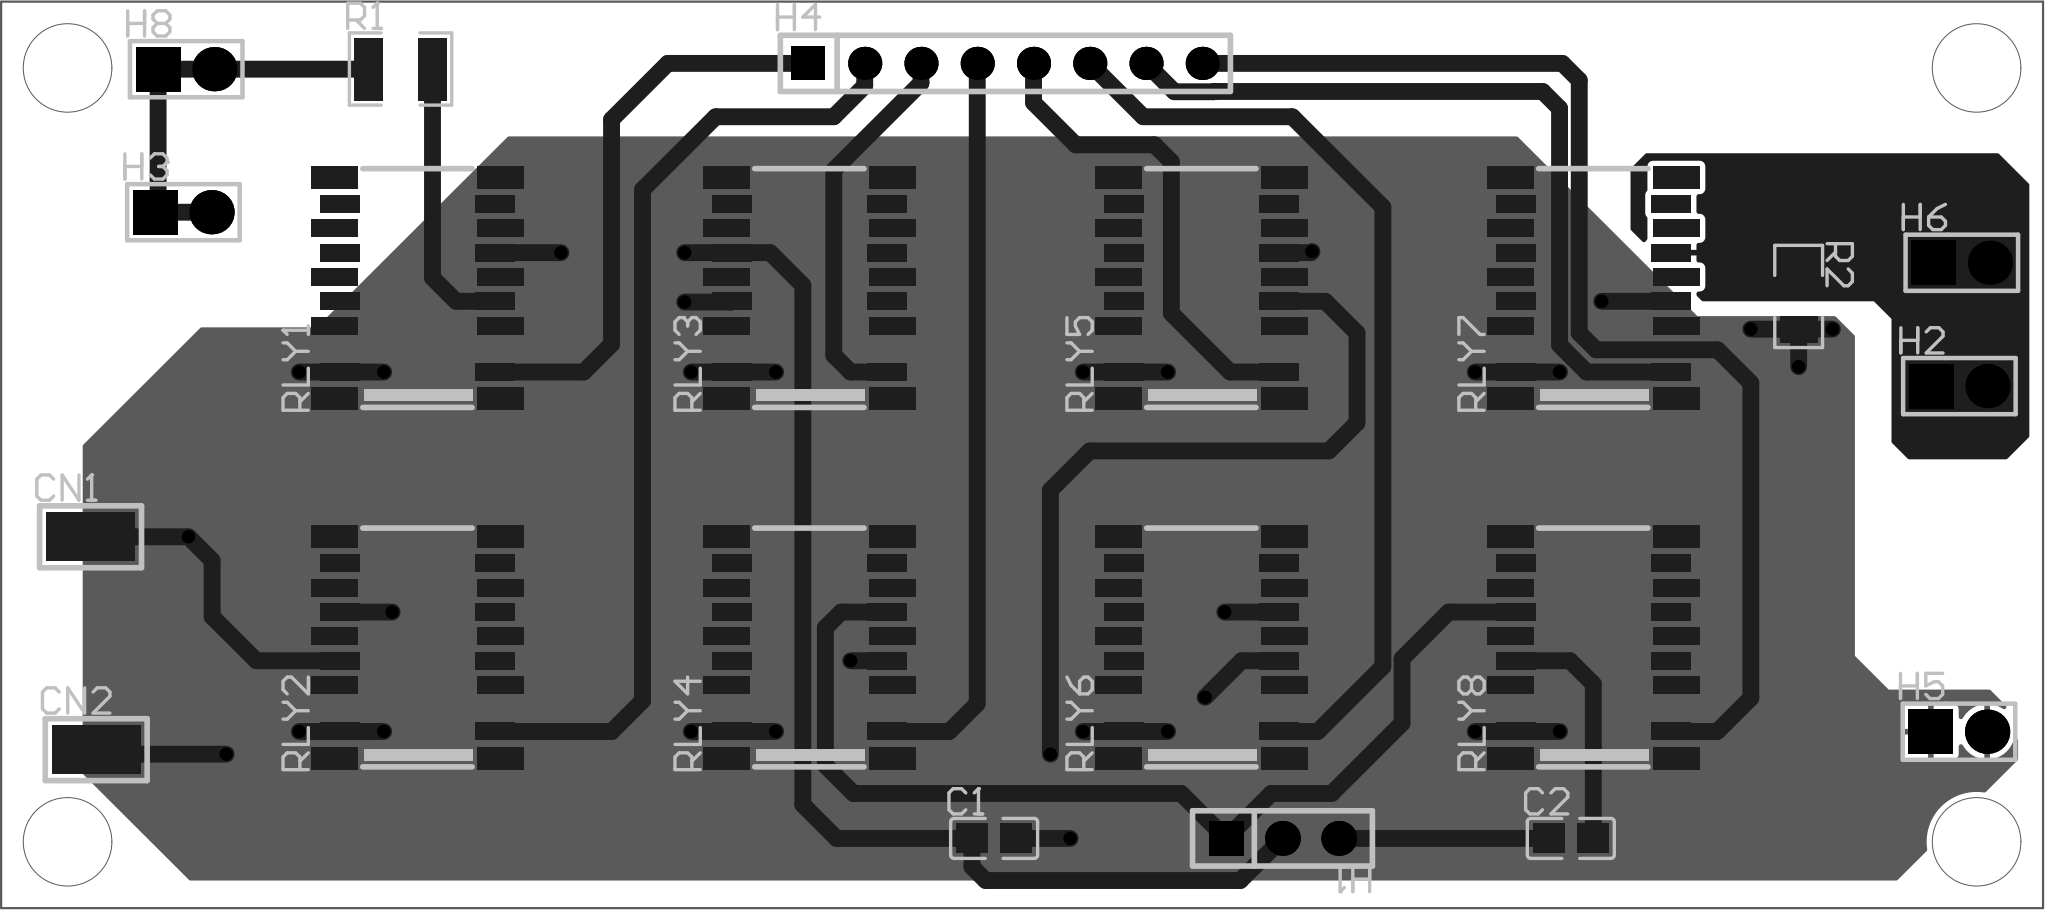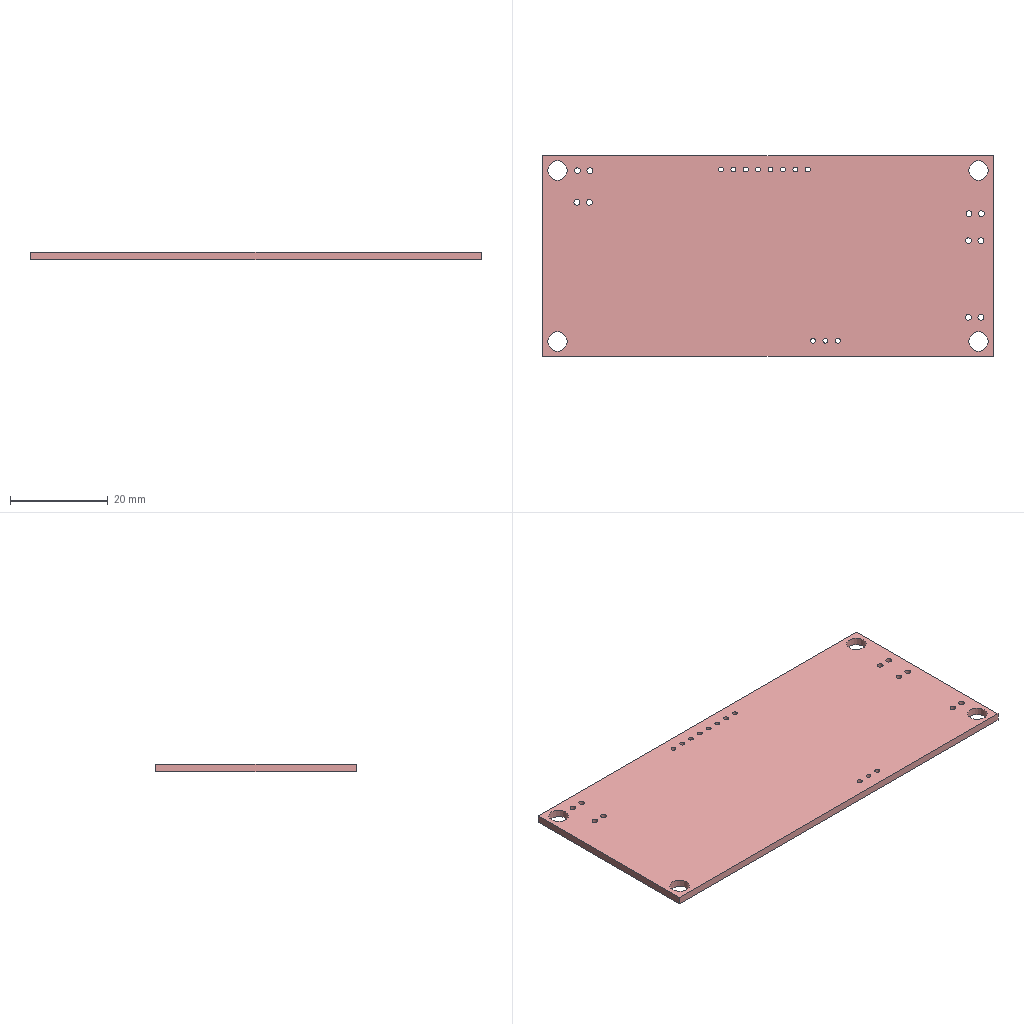Circuit board layout | Altium Designer | box 92.2 x 41 x 1.6 mm
Layer stack:
# Altium Designer layer stack of  (unit mm; dielectric type: 0 none, 1 core, 2 prepreg, 3 surface material)
index,name,kind,layer,copper_thickness_mm,dielectric_type,dielectric_thickness_mm,dielectric_material,dielectric_constant
0,Top Paste Mask Layer,other,,,,,,
1,Top Silkscreen Layer,other,,,,,,
2,Top Solder Mask Layer,dielectric,,,3,0.01,,3.3
3,Top Layer,copper,Top Layer,0.035,,,,
4,Dielectric1,dielectric,,,3,1.51,FR4,4.5
5,Bottom Layer,copper,Bottom Layer,0.035,,,,
6,Bottom Solder Mask Layer,dielectric,,,3,0.01,,3.3
7,Bottom Silkscreen Layer,other,,,,,,
8,Bottom Paste Mask Layer,other,,,,,,
# drill layer pairs: low layer,high layer
drill_pair,Top Layer,Bottom Layer
Part placement:
Designator,Comment,Layer,Footprint,Center-X(mm),Center-Y(mm),Rotation
C1,470nF,TopLayer,C0805,121.031,79.354,0
C2,470nF,TopLayer,C0805,147.066,79.354,0
CN1,RH-5019,TopLayer,TESTPOINT-SMD_L3.8-W2.0_RH-5019,80.239,92.995,0
CN2,RH-5019,TopLayer,TESTPOINT-SMD_L3.8-W2.0_RH-5019,80.493,83.368,0
H1,PM254V-11-03-H85,TopLayer,HDR-TH_3P-P2.54-V-F,134.048,79.354,0
H2,PZ254V-11-02P,TopLayer,HDR-TH_2P-P2.54-V-M,164.609,99.811,0
H3,PZ254V-11-02P,TopLayer,HDR-TH_2P-P2.54-V-M,84.43,107.675,0
H4,PZ254V-11-08P,TopLayer,HDR-TH_8P-P2.54-V-M,121.539,114.406,0
H5,PZ254V-11-02P,TopLayer,HDR-TH_2P-P2.54-V-M,164.592,84.18,0
H6,PZ254V-11-02P,TopLayer,HDR-TH_2P-P2.54-V-M,164.719,105.389,0
H8,PZ254V-11-02P,TopLayer,HDR-TH_2P-P2.54-V-M,84.557,114.144,0
R1,1kΩ,TopLayer,R1210,94.234,114.152,0
R2,0Ω,TopLayer,R1206,157.353,103.865,270
RLY1,G6K-2F-RF-S DC5,TopLayer,RELAY-SMD_G6K-2F-RF-S-DC12,94.996,104.246,90
RLY2,G6K-2F-RF-S DC5,TopLayer,RELAY-SMD_G6K-2F-RF-S-DC12,94.996,87.99,90
RLY3,G6K-2F-RF-S DC5,TopLayer,RELAY-SMD_G6K-2F-RF-S-DC12,112.691,104.246,90
RLY4,G6K-2F-RF-S DC5,TopLayer,RELAY-SMD_G6K-2F-RF-S-DC12,112.691,87.99,90
RLY5,G6K-2F-RF-S DC5,TopLayer,RELAY-SMD_G6K-2F-RF-S-DC12,130.387,104.246,90
RLY6,G6K-2F-RF-S DC5,TopLayer,RELAY-SMD_G6K-2F-RF-S-DC12,130.387,87.99,90
RLY7,G6K-2F-RF-S DC5,TopLayer,RELAY-SMD_G6K-2F-RF-S-DC12,148.082,104.246,90
RLY8,G6K-2F-RF-S DC5,TopLayer,RELAY-SMD_G6K-2F-RF-S-DC12,148.082,87.99,90
Pad and via stacks:
# Altium Designer via and pad stacks of  (unit mm). Each distinct definition once, with the count of objects using it.
# via: kind,start_layer,end_layer,hole_mm,diameter_mm,mode(0 simple;1 top-mid-bottom;2 full stack),diameter_per_layer,count,example_net
# pad: kind,layer,hole_mm,hole_type(0 round;1 square;2 slot),plating,top_size,top_shape(1 round;2 rect;3 octagon;9 rounded rect),mid_size,bottom_size,mode,footprint,size_per_layer,count,example
pad,Top Layer,0,0,plated,1.41x1.35,2,1.41x1.35,1.41x1.35,0,C0805,,4,C1.2
pad,Top Layer,0,0,plated,4x2.2,2,4x2.2,4x2.2,0,TESTPOINT-SMD_L3.8-W2.0_RH-5019,,2,CN1.1
pad,Top Layer,0,0,plated,1.282x2.808,2,1.282x2.808,1.282x2.808,0,R1210,,2,R1.2
pad,Top Layer,0,0,plated,1.208x1.701,2,1.208x1.701,1.208x1.701,0,R1206,,2,R2.2
pad,Top Layer,0,0,plated,0.8x1.8,2,0.8x1.8,0.8x1.8,0,RELAY-SMD_G6K-2F-RF-S-DC12,,64,RLY1.1
pad,Top Layer,0,0,plated,1x2.1,2,1x2.1,1x2.1,0,RELAY-SMD_G6K-2F-RF-S-DC12,,32,RLY1.9
pad,Top Layer,0,0,plated,0.8x2.1,2,0.8x2.1,0.8x2.1,0,RELAY-SMD_G6K-2F-RF-S-DC12,,48,RLY1.18
pad,Multi-Layer,1.02,0,plated,1.575x1.575,1,1.575x1.575,1.575x1.575,0,HDR-TH_3P-P2.54-V-F,,2,H1.3
pad,Multi-Layer,1.02,0,plated,1.575x1.575,2,1.575x1.575,1.575x1.575,0,HDR-TH_3P-P2.54-V-F,,1,H1.1
pad,Multi-Layer,1.2,0,plated,2x2,2,2x2,2x2,0,HDR-TH_2P-P2.54-V-M,,5,H2.1
pad,Multi-Layer,1.2,0,plated,2x2,1,2x2,2x2,0,HDR-TH_2P-P2.54-V-M,,5,H2.2
pad,Multi-Layer,1,0,plated,1.5x1.5,2,1.5x1.5,1.5x1.5,0,HDR-TH_8P-P2.54-V-M,,1,H4.1
pad,Multi-Layer,1,0,plated,1.5x1.5,1,1.5x1.5,1.5x1.5,0,HDR-TH_8P-P2.54-V-M,,7,H4.2
via,Top Layer,Bottom Layer,0.3048,0.61,0,,32,$2N20
Copper pours:
name,layer,net,type(0 solid;1 hatched;2 none)
Bottom Layer-DGND,Bottom Layer,DGND,0
Top Layer-AGND,Top Layer,AGND,0
Design rules, without the lines most boards share:
# Altium Designer design rules of  (exported by Altium Designer, unit mm)
# columns: name | kind | enabled | priority | scope1 | scope2 | descriptor | typed fields (field=value)
creepage | 65 | enabled | 1 | All | All | Creepage Distance Constraint =(0mil) (All),(All) |
copperRegion | 20 | enabled | 1 | (InNet('$2N20') OR InNet('AGND')) | All | Polygon Connect Rule(Relief Connect )(Conductor Width=10mil) (Relief Angle=90 Angle) (Entries=4) (Air Gap Width=10mil) ((InNet('$2N20') OR InNet('AGND'))),(All) | connect_style(0=relief,1=direct,2=none)=0 relief_conductor_width=0.254 relief_entries=4